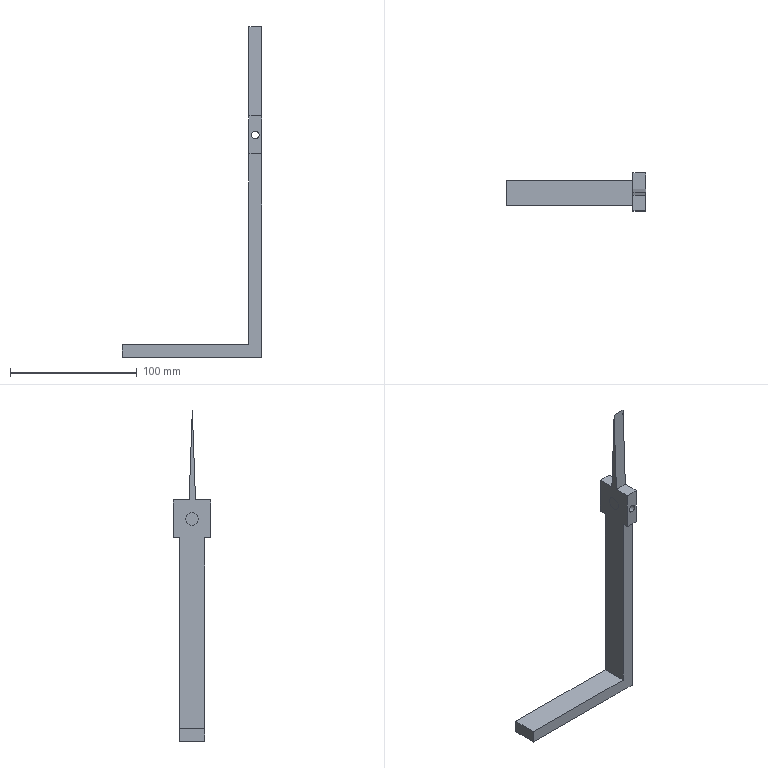Part | SolidWorks | features ICE 2, BaseBody 1 | 1 solid | 20 faces | box 110 x 30 x 261.431 mm | volume 62100 mm3 | plane 16 | cylinder 4 | commonest cylinder face diameters 6 x2 10 x2
STEP:
#1=CARTESIAN_POINT('',(-0.1,0.,44.337));
#2=VERTEX_POINT('',#1);
#3=CARTESIAN_POINT('',(-0.1,0.,34.337));
#4=VERTEX_POINT('',#3);
#5=CARTESIAN_POINT('',(-0.1,0.,39.337));
#6=DIRECTION('',(-1.,0.,0.));
#7=DIRECTION('',(0.,0.,1.));
#8=AXIS2_PLACEMENT_3D('',#5,#6,#7);
#9=CIRCLE('',#8,5.);
#10=EDGE_CURVE('',#2,#4,#9,.T.);
#11=ORIENTED_EDGE('',*,*,#10,.F.);
#12=CARTESIAN_POINT('',(0.,0.,44.337));
#13=VERTEX_POINT('',#12);
#14=CARTESIAN_POINT('',(-0.1,0.,44.337));
#15=DIRECTION('',(1.,0.,0.));
#16=VECTOR('',#15,1000.);
#17=LINE('',#14,#16);
#18=EDGE_CURVE('',#2,#13,#17,.T.);
#19=ORIENTED_EDGE('',*,*,#18,.T.);
#20=CARTESIAN_POINT('',(0.,0.,34.337));
#21=VERTEX_POINT('',#20);
#22=CARTESIAN_POINT('',(0.,0.,39.337));
#23=DIRECTION('',(-1.,0.,0.));
#24=DIRECTION('',(0.,0.,-1.));
#25=AXIS2_PLACEMENT_3D('',#22,#23,#24);
#26=CIRCLE('',#25,5.);
#27=EDGE_CURVE('',#13,#21,#26,.T.);
#28=ORIENTED_EDGE('',*,*,#27,.T.);
#29=CARTESIAN_POINT('',(-0.1,0.,34.337));
#30=DIRECTION('',(1.,0.,0.));
#31=VECTOR('',#30,1000.);
#32=LINE('',#29,#31);
#33=EDGE_CURVE('',#4,#21,#32,.T.);
#34=ORIENTED_EDGE('',*,*,#33,.F.);
#35=EDGE_LOOP('',(#11,#19,#28,#34));
#36=FACE_OUTER_BOUND('',#35,.T.);
#37=CARTESIAN_POINT('',(-0.1,0.,39.337));
#38=DIRECTION('',(1.,0.,0.));
#39=DIRECTION('',(0.,0.,-1.));
#40=AXIS2_PLACEMENT_3D('',#37,#38,#39);
#41=CYLINDRICAL_SURFACE('',#40,5.);
#42=ADVANCED_FACE('',(#36),#41,.T.);
#43=CARTESIAN_POINT('',(5.,15.,42.337));
#44=VERTEX_POINT('',#43);
#45=CARTESIAN_POINT('',(5.,15.,36.337));
#46=VERTEX_POINT('',#45);
#47=CARTESIAN_POINT('',(5.,15.,39.337));
#48=DIRECTION('',(0.,-1.,0.));
#49=DIRECTION('',(0.,0.,-1.));
#50=AXIS2_PLACEMENT_3D('',#47,#48,#49);
#51=CIRCLE('',#50,3.);
#52=EDGE_CURVE('',#44,#46,#51,.T.);
#53=ORIENTED_EDGE('',*,*,#52,.F.);
#54=CARTESIAN_POINT('',(5.,-15.,42.337));
#55=VERTEX_POINT('',#54);
#56=CARTESIAN_POINT('',(5.,15.,42.337));
#57=DIRECTION('',(0.,-1.,0.));
#58=VECTOR('',#57,1000.);
#59=LINE('',#56,#58);
#60=EDGE_CURVE('',#44,#55,#59,.T.);
#61=ORIENTED_EDGE('',*,*,#60,.T.);
#62=CARTESIAN_POINT('',(5.,-15.,36.337));
#63=VERTEX_POINT('',#62);
#64=CARTESIAN_POINT('',(5.,-15.,39.337));
#65=DIRECTION('',(0.,-1.,0.));
#66=DIRECTION('',(0.,0.,-1.));
#67=AXIS2_PLACEMENT_3D('',#64,#65,#66);
#68=CIRCLE('',#67,3.);
#69=EDGE_CURVE('',#55,#63,#68,.T.);
#70=ORIENTED_EDGE('',*,*,#69,.T.);
#71=CARTESIAN_POINT('',(5.,15.,36.337));
#72=DIRECTION('',(0.,-1.,0.));
#73=VECTOR('',#72,1000.);
#74=LINE('',#71,#73);
#75=EDGE_CURVE('',#46,#63,#74,.T.);
#76=ORIENTED_EDGE('',*,*,#75,.F.);
#77=EDGE_LOOP('',(#53,#61,#70,#76));
#78=FACE_OUTER_BOUND('',#77,.T.);
#79=CARTESIAN_POINT('',(5.,15.,39.337));
#80=DIRECTION('',(0.,-1.,0.));
#81=DIRECTION('',(0.,0.,-1.));
#82=AXIS2_PLACEMENT_3D('',#79,#80,#81);
#83=CYLINDRICAL_SURFACE('',#82,3.);
#84=ADVANCED_FACE('',(#78),#83,.F.);
#85=CARTESIAN_POINT('',(0.,0.,39.337));
#86=DIRECTION('',(-1.,0.,0.));
#87=DIRECTION('',(0.,0.,-1.));
#88=AXIS2_PLACEMENT_3D('',#85,#86,#87);
#89=CIRCLE('',#88,5.);
#90=EDGE_CURVE('',#21,#13,#89,.T.);
#91=ORIENTED_EDGE('',*,*,#90,.F.);
#92=ORIENTED_EDGE('',*,*,#27,.F.);
#93=EDGE_LOOP('',(#91,#92));
#94=FACE_BOUND('',#93,.T.);
#95=CARTESIAN_POINT('',(0.,-10.233,-126.512));
#96=VERTEX_POINT('',#95);
#97=CARTESIAN_POINT('',(0.,9.767,-126.512));
#98=VERTEX_POINT('',#97);
#99=CARTESIAN_POINT('',(0.,9.767,-126.512));
#100=DIRECTION('',(0.,1.,0.));
#101=VECTOR('',#100,1000.);
#102=LINE('',#99,#101);
#103=EDGE_CURVE('',#96,#98,#102,.T.);
#104=ORIENTED_EDGE('',*,*,#103,.F.);
#105=CARTESIAN_POINT('',(0.,-10.233,24.337));
#106=VERTEX_POINT('',#105);
#107=CARTESIAN_POINT('',(0.,-10.233,25.939));
#108=DIRECTION('',(0.,0.,-1.));
#109=VECTOR('',#108,1000.);
#110=LINE('',#107,#109);
#111=EDGE_CURVE('',#106,#96,#110,.T.);
#112=ORIENTED_EDGE('',*,*,#111,.F.);
#113=CARTESIAN_POINT('',(0.,-15.,24.337));
#114=VERTEX_POINT('',#113);
#115=CARTESIAN_POINT('',(0.,-15.,24.337));
#116=DIRECTION('',(0.,-1.,0.));
#117=VECTOR('',#116,1000.);
#118=LINE('',#115,#117);
#119=EDGE_CURVE('',#106,#114,#118,.T.);
#120=ORIENTED_EDGE('',*,*,#119,.T.);
#121=CARTESIAN_POINT('',(0.,-15.,54.337));
#122=VERTEX_POINT('',#121);
#123=CARTESIAN_POINT('',(0.,-15.,54.337));
#124=DIRECTION('',(0.,0.,-1.));
#125=VECTOR('',#124,1000.);
#126=LINE('',#123,#125);
#127=EDGE_CURVE('',#122,#114,#126,.T.);
#128=ORIENTED_EDGE('',*,*,#127,.F.);
#129=CARTESIAN_POINT('',(0.,-2.742,54.337));
#130=VERTEX_POINT('',#129);
#131=CARTESIAN_POINT('',(0.,2.277,54.337));
#132=DIRECTION('',(0.,1.,0.));
#133=VECTOR('',#132,1000.);
#134=LINE('',#131,#133);
#135=EDGE_CURVE('',#122,#130,#134,.T.);
#136=ORIENTED_EDGE('',*,*,#135,.T.);
#137=CARTESIAN_POINT('',(0.,-0.2326,124.919));
#138=VERTEX_POINT('',#137);
#139=CARTESIAN_POINT('',(0.,-0.2326,124.919));
#140=DIRECTION('',(0.,0.03553,0.9994));
#141=VECTOR('',#140,1000.);
#142=LINE('',#139,#141);
#143=EDGE_CURVE('',#130,#138,#142,.T.);
#144=ORIENTED_EDGE('',*,*,#143,.T.);
#145=CARTESIAN_POINT('',(0.,2.277,54.337));
#146=VERTEX_POINT('',#145);
#147=CARTESIAN_POINT('',(0.,-0.2326,124.919));
#148=DIRECTION('',(0.,0.03553,-0.9994));
#149=VECTOR('',#148,1000.);
#150=LINE('',#147,#149);
#151=EDGE_CURVE('',#138,#146,#150,.T.);
#152=ORIENTED_EDGE('',*,*,#151,.T.);
#153=CARTESIAN_POINT('',(0.,15.,54.337));
#154=VERTEX_POINT('',#153);
#155=CARTESIAN_POINT('',(0.,2.277,54.337));
#156=DIRECTION('',(0.,1.,0.));
#157=VECTOR('',#156,1000.);
#158=LINE('',#155,#157);
#159=EDGE_CURVE('',#146,#154,#158,.T.);
#160=ORIENTED_EDGE('',*,*,#159,.T.);
#161=CARTESIAN_POINT('',(0.,15.,24.337));
#162=VERTEX_POINT('',#161);
#163=CARTESIAN_POINT('',(0.,15.,54.337));
#164=DIRECTION('',(0.,0.,1.));
#165=VECTOR('',#164,1000.);
#166=LINE('',#163,#165);
#167=EDGE_CURVE('',#162,#154,#166,.T.);
#168=ORIENTED_EDGE('',*,*,#167,.F.);
#169=CARTESIAN_POINT('',(0.,9.767,24.337));
#170=VERTEX_POINT('',#169);
#171=CARTESIAN_POINT('',(0.,-15.,24.337));
#172=DIRECTION('',(0.,-1.,0.));
#173=VECTOR('',#172,1000.);
#174=LINE('',#171,#173);
#175=EDGE_CURVE('',#162,#170,#174,.T.);
#176=ORIENTED_EDGE('',*,*,#175,.T.);
#177=CARTESIAN_POINT('',(0.,9.767,25.939));
#178=DIRECTION('',(0.,0.,1.));
#179=VECTOR('',#178,1000.);
#180=LINE('',#177,#179);
#181=EDGE_CURVE('',#98,#170,#180,.T.);
#182=ORIENTED_EDGE('',*,*,#181,.F.);
#183=EDGE_LOOP('',(#104,#112,#120,#128,#136,#144,#152,#160,#168,#176,#182));
#184=FACE_OUTER_BOUND('',#183,.T.);
#185=CARTESIAN_POINT('',(0.,-0.2326,38.488));
#186=DIRECTION('',(1.,0.,0.));
#187=DIRECTION('',(0.,0.,-1.));
#188=AXIS2_PLACEMENT_3D('',#185,#186,#187);
#189=PLANE('',#188);
#190=ADVANCED_FACE('',(#94,#184),#189,.F.);
#191=CARTESIAN_POINT('',(-100.,-10.233,-136.512));
#192=VERTEX_POINT('',#191);
#193=CARTESIAN_POINT('',(-100.,-10.233,-126.512));
#194=VERTEX_POINT('',#193);
#195=CARTESIAN_POINT('',(-100.,-10.233,-141.512));
#196=DIRECTION('',(0.,0.,1.));
#197=VECTOR('',#196,1000.);
#198=LINE('',#195,#197);
#199=EDGE_CURVE('',#192,#194,#198,.T.);
#200=ORIENTED_EDGE('',*,*,#199,.F.);
#201=CARTESIAN_POINT('',(10.,-10.233,-136.512));
#202=VERTEX_POINT('',#201);
#203=CARTESIAN_POINT('',(-100.,-10.233,-136.512));
#204=DIRECTION('',(-1.,0.,0.));
#205=VECTOR('',#204,1000.);
#206=LINE('',#203,#205);
#207=EDGE_CURVE('',#202,#192,#206,.T.);
#208=ORIENTED_EDGE('',*,*,#207,.F.);
#209=CARTESIAN_POINT('',(10.,-10.233,24.337));
#210=VERTEX_POINT('',#209);
#211=CARTESIAN_POINT('',(10.,-10.233,25.939));
#212=DIRECTION('',(0.,0.,-1.));
#213=VECTOR('',#212,1000.);
#214=LINE('',#211,#213);
#215=EDGE_CURVE('',#210,#202,#214,.T.);
#216=ORIENTED_EDGE('',*,*,#215,.F.);
#217=CARTESIAN_POINT('',(10.,-10.233,24.337));
#218=DIRECTION('',(-1.,0.,0.));
#219=VECTOR('',#218,1000.);
#220=LINE('',#217,#219);
#221=EDGE_CURVE('',#210,#106,#220,.T.);
#222=ORIENTED_EDGE('',*,*,#221,.T.);
#223=ORIENTED_EDGE('',*,*,#111,.T.);
#224=CARTESIAN_POINT('',(0.,-10.233,-126.512));
#225=DIRECTION('',(1.,0.,0.));
#226=VECTOR('',#225,1000.);
#227=LINE('',#224,#226);
#228=EDGE_CURVE('',#194,#96,#227,.T.);
#229=ORIENTED_EDGE('',*,*,#228,.F.);
#230=EDGE_LOOP('',(#200,#208,#216,#222,#223,#229));
#231=FACE_OUTER_BOUND('',#230,.T.);
#232=CARTESIAN_POINT('',(10.,-10.233,25.939));
#233=DIRECTION('',(0.,1.,0.));
#234=DIRECTION('',(0.,0.,1.));
#235=AXIS2_PLACEMENT_3D('',#232,#233,#234);
#236=PLANE('',#235);
#237=ADVANCED_FACE('',(#231),#236,.F.);
#238=CARTESIAN_POINT('',(-100.,9.767,-126.512));
#239=VERTEX_POINT('',#238);
#240=CARTESIAN_POINT('',(-100.,9.767,-126.512));
#241=DIRECTION('',(-1.,0.,0.));
#242=VECTOR('',#241,1000.);
#243=LINE('',#240,#242);
#244=EDGE_CURVE('',#98,#239,#243,.T.);
#245=ORIENTED_EDGE('',*,*,#244,.F.);
#246=ORIENTED_EDGE('',*,*,#181,.T.);
#247=CARTESIAN_POINT('',(10.,9.767,24.337));
#248=VERTEX_POINT('',#247);
#249=CARTESIAN_POINT('',(10.,9.767,24.337));
#250=DIRECTION('',(1.,0.,0.));
#251=VECTOR('',#250,1000.);
#252=LINE('',#249,#251);
#253=EDGE_CURVE('',#170,#248,#252,.T.);
#254=ORIENTED_EDGE('',*,*,#253,.T.);
#255=CARTESIAN_POINT('',(10.,9.767,-136.512));
#256=VERTEX_POINT('',#255);
#257=CARTESIAN_POINT('',(10.,9.767,25.939));
#258=DIRECTION('',(0.,0.,1.));
#259=VECTOR('',#258,1000.);
#260=LINE('',#257,#259);
#261=EDGE_CURVE('',#256,#248,#260,.T.);
#262=ORIENTED_EDGE('',*,*,#261,.F.);
#263=CARTESIAN_POINT('',(-100.,9.767,-136.512));
#264=VERTEX_POINT('',#263);
#265=CARTESIAN_POINT('',(10.,9.767,-136.512));
#266=DIRECTION('',(1.,0.,0.));
#267=VECTOR('',#266,1000.);
#268=LINE('',#265,#267);
#269=EDGE_CURVE('',#264,#256,#268,.T.);
#270=ORIENTED_EDGE('',*,*,#269,.F.);
#271=CARTESIAN_POINT('',(-100.,9.767,-141.512));
#272=DIRECTION('',(0.,0.,1.));
#273=VECTOR('',#272,1000.);
#274=LINE('',#271,#273);
#275=EDGE_CURVE('',#264,#239,#274,.T.);
#276=ORIENTED_EDGE('',*,*,#275,.T.);
#277=EDGE_LOOP('',(#245,#246,#254,#262,#270,#276));
#278=FACE_OUTER_BOUND('',#277,.T.);
#279=CARTESIAN_POINT('',(10.,9.767,25.939));
#280=DIRECTION('',(0.,-1.,0.));
#281=DIRECTION('',(0.,0.,-1.));
#282=AXIS2_PLACEMENT_3D('',#279,#280,#281);
#283=PLANE('',#282);
#284=ADVANCED_FACE('',(#278),#283,.F.);
#285=CARTESIAN_POINT('',(10.,-10.233,-136.512));
#286=DIRECTION('',(0.,-1.,0.));
#287=VECTOR('',#286,1000.);
#288=LINE('',#285,#287);
#289=EDGE_CURVE('',#256,#202,#288,.T.);
#290=ORIENTED_EDGE('',*,*,#289,.F.);
#291=ORIENTED_EDGE('',*,*,#261,.T.);
#292=CARTESIAN_POINT('',(10.,15.,24.337));
#293=VERTEX_POINT('',#292);
#294=CARTESIAN_POINT('',(10.,-15.,24.337));
#295=DIRECTION('',(0.,-1.,0.));
#296=VECTOR('',#295,1000.);
#297=LINE('',#294,#296);
#298=EDGE_CURVE('',#293,#248,#297,.T.);
#299=ORIENTED_EDGE('',*,*,#298,.F.);
#300=CARTESIAN_POINT('',(10.,15.,54.337));
#301=VERTEX_POINT('',#300);
#302=CARTESIAN_POINT('',(10.,15.,54.337));
#303=DIRECTION('',(0.,0.,1.));
#304=VECTOR('',#303,1000.);
#305=LINE('',#302,#304);
#306=EDGE_CURVE('',#293,#301,#305,.T.);
#307=ORIENTED_EDGE('',*,*,#306,.T.);
#308=CARTESIAN_POINT('',(10.,2.277,54.337));
#309=VERTEX_POINT('',#308);
#310=CARTESIAN_POINT('',(10.,-16.764,54.337));
#311=DIRECTION('',(0.,1.,0.));
#312=VECTOR('',#311,1000.);
#313=LINE('',#310,#312);
#314=EDGE_CURVE('',#309,#301,#313,.T.);
#315=ORIENTED_EDGE('',*,*,#314,.F.);
#316=CARTESIAN_POINT('',(10.,-0.2326,124.919));
#317=VERTEX_POINT('',#316);
#318=CARTESIAN_POINT('',(10.,-0.2326,124.919));
#319=DIRECTION('',(0.,-0.03553,0.9994));
#320=VECTOR('',#319,1000.);
#321=LINE('',#318,#320);
#322=EDGE_CURVE('',#309,#317,#321,.T.);
#323=ORIENTED_EDGE('',*,*,#322,.T.);
#324=CARTESIAN_POINT('',(10.,-2.742,54.337));
#325=VERTEX_POINT('',#324);
#326=CARTESIAN_POINT('',(10.,-0.2326,124.919));
#327=DIRECTION('',(0.,-0.03553,-0.9994));
#328=VECTOR('',#327,1000.);
#329=LINE('',#326,#328);
#330=EDGE_CURVE('',#317,#325,#329,.T.);
#331=ORIENTED_EDGE('',*,*,#330,.T.);
#332=CARTESIAN_POINT('',(10.,-15.,54.337));
#333=VERTEX_POINT('',#332);
#334=CARTESIAN_POINT('',(10.,-16.764,54.337));
#335=DIRECTION('',(0.,1.,0.));
#336=VECTOR('',#335,1000.);
#337=LINE('',#334,#336);
#338=EDGE_CURVE('',#333,#325,#337,.T.);
#339=ORIENTED_EDGE('',*,*,#338,.F.);
#340=CARTESIAN_POINT('',(10.,-15.,24.337));
#341=VERTEX_POINT('',#340);
#342=CARTESIAN_POINT('',(10.,-15.,54.337));
#343=DIRECTION('',(0.,0.,-1.));
#344=VECTOR('',#343,1000.);
#345=LINE('',#342,#344);
#346=EDGE_CURVE('',#333,#341,#345,.T.);
#347=ORIENTED_EDGE('',*,*,#346,.T.);
#348=CARTESIAN_POINT('',(10.,-15.,24.337));
#349=DIRECTION('',(0.,-1.,0.));
#350=VECTOR('',#349,1000.);
#351=LINE('',#348,#350);
#352=EDGE_CURVE('',#210,#341,#351,.T.);
#353=ORIENTED_EDGE('',*,*,#352,.F.);
#354=ORIENTED_EDGE('',*,*,#215,.T.);
#355=EDGE_LOOP('',(#290,#291,#299,#307,#315,#323,#331,#339,#347,#353,#354));
#356=FACE_OUTER_BOUND('',#355,.T.);
#357=CARTESIAN_POINT('',(10.,-0.2326,38.488));
#358=DIRECTION('',(1.,0.,0.));
#359=DIRECTION('',(0.,0.,-1.));
#360=AXIS2_PLACEMENT_3D('',#357,#358,#359);
#361=PLANE('',#360);
#362=ADVANCED_FACE('',(#356),#361,.T.);
#363=ORIENTED_EDGE('',*,*,#151,.F.);
#364=CARTESIAN_POINT('',(-72.43,-0.2326,124.919));
#365=DIRECTION('',(1.,0.,0.));
#366=VECTOR('',#365,1000.);
#367=LINE('',#364,#366);
#368=EDGE_CURVE('',#138,#317,#367,.T.);
#369=ORIENTED_EDGE('',*,*,#368,.T.);
#370=ORIENTED_EDGE('',*,*,#322,.F.);
#371=CARTESIAN_POINT('',(-72.43,2.277,54.337));
#372=DIRECTION('',(1.,0.,0.));
#373=VECTOR('',#372,1000.);
#374=LINE('',#371,#373);
#375=EDGE_CURVE('',#146,#309,#374,.T.);
#376=ORIENTED_EDGE('',*,*,#375,.F.);
#377=EDGE_LOOP('',(#363,#369,#370,#376));
#378=FACE_OUTER_BOUND('',#377,.T.);
#379=CARTESIAN_POINT('',(-72.43,-0.2326,124.919));
#380=DIRECTION('',(0.,0.9994,0.03553));
#381=DIRECTION('',(0.,-0.03553,0.9994));
#382=AXIS2_PLACEMENT_3D('',#379,#380,#381);
#383=PLANE('',#382);
#384=ADVANCED_FACE('',(#378),#383,.T.);
#385=ORIENTED_EDGE('',*,*,#143,.F.);
#386=CARTESIAN_POINT('',(-72.43,-2.742,54.337));
#387=DIRECTION('',(1.,0.,0.));
#388=VECTOR('',#387,1000.);
#389=LINE('',#386,#388);
#390=EDGE_CURVE('',#130,#325,#389,.T.);
#391=ORIENTED_EDGE('',*,*,#390,.T.);
#392=ORIENTED_EDGE('',*,*,#330,.F.);
#393=ORIENTED_EDGE('',*,*,#368,.F.);
#394=EDGE_LOOP('',(#385,#391,#392,#393));
#395=FACE_OUTER_BOUND('',#394,.T.);
#396=CARTESIAN_POINT('',(-72.43,-0.2326,124.919));
#397=DIRECTION('',(0.,-0.9994,0.03553));
#398=DIRECTION('',(0.,-0.03553,-0.9994));
#399=AXIS2_PLACEMENT_3D('',#396,#397,#398);
#400=PLANE('',#399);
#401=ADVANCED_FACE('',(#395),#400,.T.);
#402=ORIENTED_EDGE('',*,*,#275,.F.);
#403=CARTESIAN_POINT('',(-100.,9.767,-136.512));
#404=DIRECTION('',(0.,1.,0.));
#405=VECTOR('',#404,1000.);
#406=LINE('',#403,#405);
#407=EDGE_CURVE('',#192,#264,#406,.T.);
#408=ORIENTED_EDGE('',*,*,#407,.F.);
#409=ORIENTED_EDGE('',*,*,#199,.T.);
#410=CARTESIAN_POINT('',(-100.,-10.233,-126.512));
#411=DIRECTION('',(0.,-1.,0.));
#412=VECTOR('',#411,1000.);
#413=LINE('',#410,#412);
#414=EDGE_CURVE('',#239,#194,#413,.T.);
#415=ORIENTED_EDGE('',*,*,#414,.F.);
#416=EDGE_LOOP('',(#402,#408,#409,#415));
#417=FACE_OUTER_BOUND('',#416,.T.);
#418=CARTESIAN_POINT('',(-100.,0.,0.));
#419=DIRECTION('',(1.,0.,0.));
#420=DIRECTION('',(0.,0.,-1.));
#421=AXIS2_PLACEMENT_3D('',#418,#419,#420);
#422=PLANE('',#421);
#423=ADVANCED_FACE('',(#417),#422,.F.);
#424=CARTESIAN_POINT('',(10.,-15.,54.337));
#425=DIRECTION('',(-1.,0.,0.));
#426=VECTOR('',#425,1000.);
#427=LINE('',#424,#426);
#428=EDGE_CURVE('',#333,#122,#427,.T.);
#429=ORIENTED_EDGE('',*,*,#428,.F.);
#430=ORIENTED_EDGE('',*,*,#338,.T.);
#431=ORIENTED_EDGE('',*,*,#390,.F.);
#432=ORIENTED_EDGE('',*,*,#135,.F.);
#433=EDGE_LOOP('',(#429,#430,#431,#432));
#434=FACE_OUTER_BOUND('',#433,.T.);
#435=CARTESIAN_POINT('',(10.,2.277,54.337));
#436=DIRECTION('',(0.,0.,1.));
#437=DIRECTION('',(1.,0.,0.));
#438=AXIS2_PLACEMENT_3D('',#435,#436,#437);
#439=PLANE('',#438);
#440=ADVANCED_FACE('',(#434),#439,.T.);
#441=CARTESIAN_POINT('',(10.,15.,54.337));
#442=DIRECTION('',(-1.,0.,0.));
#443=VECTOR('',#442,1000.);
#444=LINE('',#441,#443);
#445=EDGE_CURVE('',#301,#154,#444,.T.);
#446=ORIENTED_EDGE('',*,*,#445,.T.);
#447=ORIENTED_EDGE('',*,*,#159,.F.);
#448=ORIENTED_EDGE('',*,*,#375,.T.);
#449=ORIENTED_EDGE('',*,*,#314,.T.);
#450=EDGE_LOOP('',(#446,#447,#448,#449));
#451=FACE_OUTER_BOUND('',#450,.T.);
#452=CARTESIAN_POINT('',(10.,2.277,54.337));
#453=DIRECTION('',(0.,0.,1.));
#454=DIRECTION('',(1.,0.,0.));
#455=AXIS2_PLACEMENT_3D('',#452,#453,#454);
#456=PLANE('',#455);
#457=ADVANCED_FACE('',(#451),#456,.T.);
#458=CARTESIAN_POINT('',(5.,15.,39.337));
#459=DIRECTION('',(0.,-1.,0.));
#460=DIRECTION('',(0.,0.,-1.));
#461=AXIS2_PLACEMENT_3D('',#458,#459,#460);
#462=CIRCLE('',#461,3.);
#463=EDGE_CURVE('',#46,#44,#462,.T.);
#464=ORIENTED_EDGE('',*,*,#463,.T.);
#465=ORIENTED_EDGE('',*,*,#52,.T.);
#466=EDGE_LOOP('',(#464,#465));
#467=FACE_BOUND('',#466,.T.);
#468=ORIENTED_EDGE('',*,*,#167,.T.);
#469=ORIENTED_EDGE('',*,*,#445,.F.);
#470=ORIENTED_EDGE('',*,*,#306,.F.);
#471=CARTESIAN_POINT('',(10.,15.,24.337));
#472=DIRECTION('',(-1.,0.,0.));
#473=VECTOR('',#472,1000.);
#474=LINE('',#471,#473);
#475=EDGE_CURVE('',#293,#162,#474,.T.);
#476=ORIENTED_EDGE('',*,*,#475,.T.);
#477=EDGE_LOOP('',(#468,#469,#470,#476));
#478=FACE_OUTER_BOUND('',#477,.T.);
#479=CARTESIAN_POINT('',(10.,15.,54.337));
#480=DIRECTION('',(0.,-1.,0.));
#481=DIRECTION('',(0.,0.,-1.));
#482=AXIS2_PLACEMENT_3D('',#479,#480,#481);
#483=PLANE('',#482);
#484=ADVANCED_FACE('',(#467,#478),#483,.F.);
#485=CARTESIAN_POINT('',(5.,-15.,39.337));
#486=DIRECTION('',(0.,-1.,0.));
#487=DIRECTION('',(0.,0.,-1.));
#488=AXIS2_PLACEMENT_3D('',#485,#486,#487);
#489=CIRCLE('',#488,3.);
#490=EDGE_CURVE('',#63,#55,#489,.T.);
#491=ORIENTED_EDGE('',*,*,#490,.F.);
#492=ORIENTED_EDGE('',*,*,#69,.F.);
#493=EDGE_LOOP('',(#491,#492));
#494=FACE_BOUND('',#493,.T.);
#495=ORIENTED_EDGE('',*,*,#127,.T.);
#496=CARTESIAN_POINT('',(10.,-15.,24.337));
#497=DIRECTION('',(-1.,0.,0.));
#498=VECTOR('',#497,1000.);
#499=LINE('',#496,#498);
#500=EDGE_CURVE('',#341,#114,#499,.T.);
#501=ORIENTED_EDGE('',*,*,#500,.F.);
#502=ORIENTED_EDGE('',*,*,#346,.F.);
#503=ORIENTED_EDGE('',*,*,#428,.T.);
#504=EDGE_LOOP('',(#495,#501,#502,#503));
#505=FACE_OUTER_BOUND('',#504,.T.);
#506=CARTESIAN_POINT('',(10.,-15.,54.337));
#507=DIRECTION('',(0.,1.,0.));
#508=DIRECTION('',(0.,0.,1.));
#509=AXIS2_PLACEMENT_3D('',#506,#507,#508);
#510=PLANE('',#509);
#511=ADVANCED_FACE('',(#494,#505),#510,.F.);
#512=ORIENTED_EDGE('',*,*,#221,.F.);
#513=ORIENTED_EDGE('',*,*,#352,.T.);
#514=ORIENTED_EDGE('',*,*,#500,.T.);
#515=ORIENTED_EDGE('',*,*,#119,.F.);
#516=EDGE_LOOP('',(#512,#513,#514,#515));
#517=FACE_OUTER_BOUND('',#516,.T.);
#518=CARTESIAN_POINT('',(10.,-15.,24.337));
#519=DIRECTION('',(0.,0.,-1.));
#520=DIRECTION('',(-1.,0.,0.));
#521=AXIS2_PLACEMENT_3D('',#518,#519,#520);
#522=PLANE('',#521);
#523=ADVANCED_FACE('',(#517),#522,.T.);
#524=ORIENTED_EDGE('',*,*,#253,.F.);
#525=ORIENTED_EDGE('',*,*,#175,.F.);
#526=ORIENTED_EDGE('',*,*,#475,.F.);
#527=ORIENTED_EDGE('',*,*,#298,.T.);
#528=EDGE_LOOP('',(#524,#525,#526,#527));
#529=FACE_OUTER_BOUND('',#528,.T.);
#530=CARTESIAN_POINT('',(10.,-15.,24.337));
#531=DIRECTION('',(0.,0.,-1.));
#532=DIRECTION('',(-1.,0.,0.));
#533=AXIS2_PLACEMENT_3D('',#530,#531,#532);
#534=PLANE('',#533);
#535=ADVANCED_FACE('',(#529),#534,.T.);
#536=ORIENTED_EDGE('',*,*,#60,.F.);
#537=ORIENTED_EDGE('',*,*,#463,.F.);
#538=ORIENTED_EDGE('',*,*,#75,.T.);
#539=ORIENTED_EDGE('',*,*,#490,.T.);
#540=EDGE_LOOP('',(#536,#537,#538,#539));
#541=FACE_OUTER_BOUND('',#540,.T.);
#542=CARTESIAN_POINT('',(5.,15.,39.337));
#543=DIRECTION('',(0.,-1.,0.));
#544=DIRECTION('',(0.,0.,-1.));
#545=AXIS2_PLACEMENT_3D('',#542,#543,#544);
#546=CYLINDRICAL_SURFACE('',#545,3.);
#547=ADVANCED_FACE('',(#541),#546,.F.);
#548=ORIENTED_EDGE('',*,*,#18,.F.);
#549=CARTESIAN_POINT('',(-0.1,0.,39.337));
#550=DIRECTION('',(-1.,0.,0.));
#551=DIRECTION('',(0.,0.,1.));
#552=AXIS2_PLACEMENT_3D('',#549,#550,#551);
#553=CIRCLE('',#552,5.);
#554=EDGE_CURVE('',#4,#2,#553,.T.);
#555=ORIENTED_EDGE('',*,*,#554,.F.);
#556=ORIENTED_EDGE('',*,*,#33,.T.);
#557=ORIENTED_EDGE('',*,*,#90,.T.);
#558=EDGE_LOOP('',(#548,#555,#556,#557));
#559=FACE_OUTER_BOUND('',#558,.T.);
#560=CARTESIAN_POINT('',(-0.1,0.,39.337));
#561=DIRECTION('',(1.,0.,0.));
#562=DIRECTION('',(0.,0.,-1.));
#563=AXIS2_PLACEMENT_3D('',#560,#561,#562);
#564=CYLINDRICAL_SURFACE('',#563,5.);
#565=ADVANCED_FACE('',(#559),#564,.T.);
#566=ORIENTED_EDGE('',*,*,#554,.T.);
#567=ORIENTED_EDGE('',*,*,#10,.T.);
#568=EDGE_LOOP('',(#566,#567));
#569=FACE_OUTER_BOUND('',#568,.T.);
#570=CARTESIAN_POINT('',(-0.1,0.,39.337));
#571=DIRECTION('',(-1.,0.,0.));
#572=DIRECTION('',(0.,0.,1.));
#573=AXIS2_PLACEMENT_3D('',#570,#571,#572);
#574=PLANE('',#573);
#575=ADVANCED_FACE('',(#569),#574,.T.);
#576=ORIENTED_EDGE('',*,*,#289,.T.);
#577=ORIENTED_EDGE('',*,*,#207,.T.);
#578=ORIENTED_EDGE('',*,*,#407,.T.);
#579=ORIENTED_EDGE('',*,*,#269,.T.);
#580=EDGE_LOOP('',(#576,#577,#578,#579));
#581=FACE_OUTER_BOUND('',#580,.T.);
#582=CARTESIAN_POINT('',(0.,0.,-136.512));
#583=DIRECTION('',(0.,0.,1.));
#584=DIRECTION('',(1.,0.,0.));
#585=AXIS2_PLACEMENT_3D('',#582,#583,#584);
#586=PLANE('',#585);
#587=ADVANCED_FACE('',(#581),#586,.F.);
#588=ORIENTED_EDGE('',*,*,#414,.T.);
#589=ORIENTED_EDGE('',*,*,#228,.T.);
#590=ORIENTED_EDGE('',*,*,#103,.T.);
#591=ORIENTED_EDGE('',*,*,#244,.T.);
#592=EDGE_LOOP('',(#588,#589,#590,#591));
#593=FACE_OUTER_BOUND('',#592,.T.);
#594=CARTESIAN_POINT('',(0.,0.,-126.512));
#595=DIRECTION('',(0.,0.,-1.));
#596=DIRECTION('',(-1.,0.,0.));
#597=AXIS2_PLACEMENT_3D('',#594,#595,#596);
#598=PLANE('',#597);
#599=ADVANCED_FACE('',(#593),#598,.F.);
#600=CLOSED_SHELL('',(#42,#84,#190,#237,#284,#362,#384,#401,#423,#440,#457,#484,#511,#523,#535,#547,#565,#575,#587,#599));
#601=MANIFOLD_SOLID_BREP('',#600);
#602=CARTESIAN_POINT('',(0.,0.,0.));
#603=DIRECTION('',(0.,0.,1.));
#604=DIRECTION('',(1.,0.,0.));
#605=AXIS2_PLACEMENT_3D('',#602,#603,#604);
#606=(LENGTH_UNIT()NAMED_UNIT(*)SI_UNIT(.MILLI.,.METRE.));
#607=UNCERTAINTY_MEASURE_WITH_UNIT(LENGTH_MEASURE(0.00001),#606,'','');
#608=(NAMED_UNIT(*)PLANE_ANGLE_UNIT()SI_UNIT($,.RADIAN.));
#609=(NAMED_UNIT(*)SI_UNIT($,.STERADIAN.)SOLID_ANGLE_UNIT());
#610=(GEOMETRIC_REPRESENTATION_CONTEXT(3)GLOBAL_UNCERTAINTY_ASSIGNED_CONTEXT((#607))GLOBAL_UNIT_ASSIGNED_CONTEXT((#606,#608,#609))REPRESENTATION_CONTEXT('',''));
#611=ADVANCED_BREP_SHAPE_REPRESENTATION('',(#601,#605),#610);